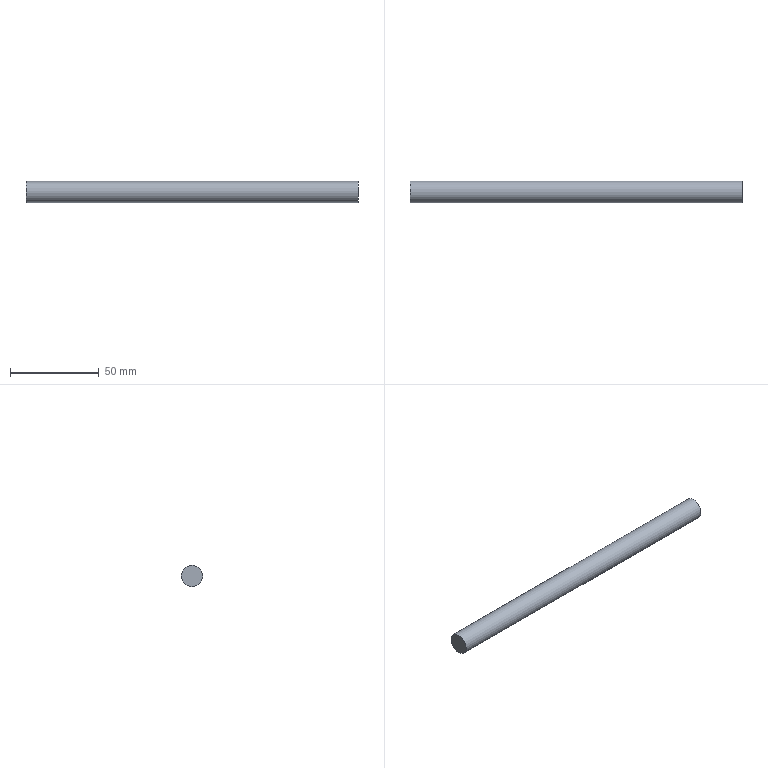Part | STEP file | solid 110 | 1 solid | 3 faces | box 187 x 12 x 12 mm | volume 21149 mm3 | plane 2 | cylinder 1 | commonest cylinder face diameters 12 x1